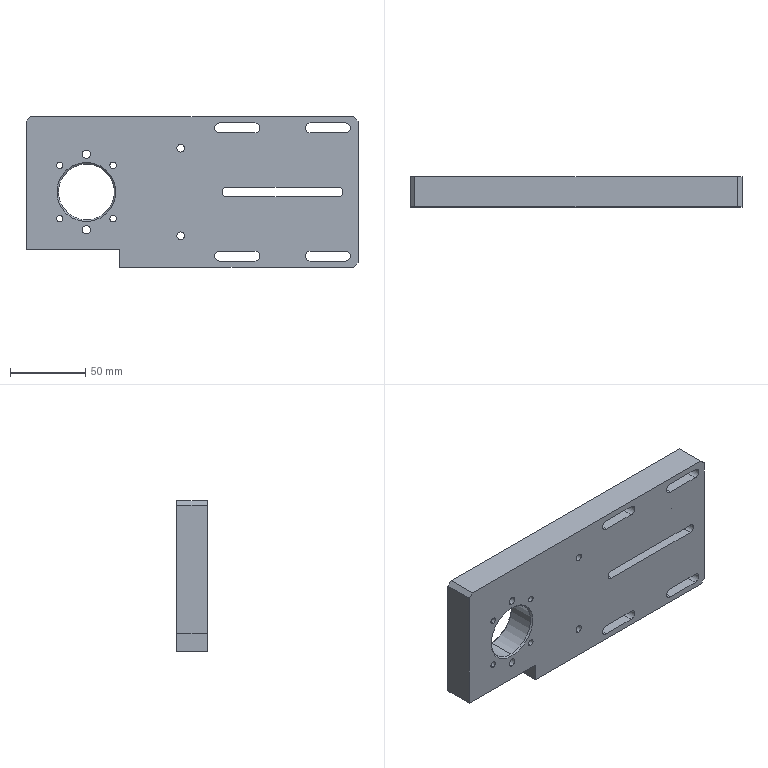Part | SolidWorks | features HoleWzd 11, Chamfer 2, ICE 2, Cut 1, Extrusion 1 | 1 solid | 121 faces | box 220 x 20 x 100 mm | volume 365463 mm3 | cylinder 60 | plane 33 | cone 28 | commonest cylinder face diameters 4.2 x12 6 x10 5 x8 6.6 x8 11 x8 3.3 x4